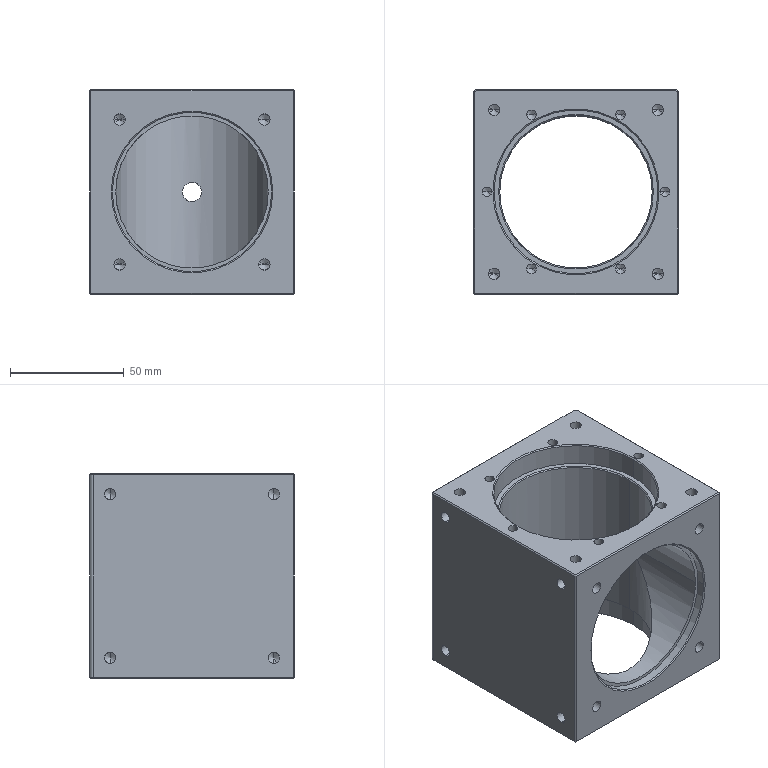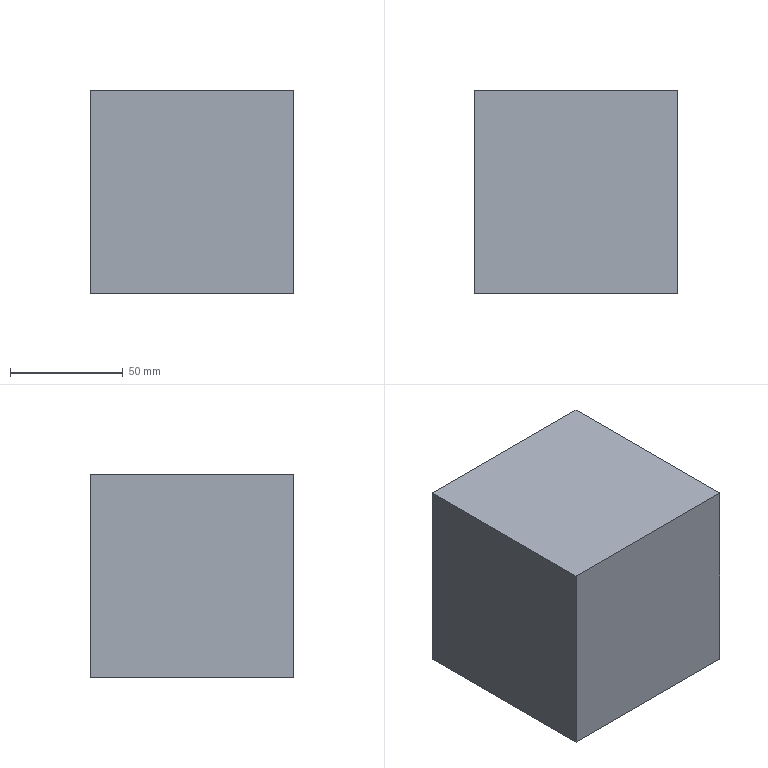CAM job | NX | 3+2 milling, drilling | part box 90 x 90 x 90 mm | stock box 90 x 90 x 90 mm
Tools:
number,name,description,diameter,corner_radius,flute_length,length,flutes
7,D6A45,Milling Tool-5 Parameters,6.0,0.0,3.0,3.0,2
14,4.2ZT,Drilling Tool,4.2,0.0,35.0,50.0,2
15,5.0ZT,Drilling Tool,5.0,0.0,35.0,50.0,2
9,9.0ZT,Drilling Tool,9.0,0.0,35.0,50.0,2
10,D10,Milling Tool-5 Parameters,10.0,0.0,50.0,75.0,2
16,D16,Milling Tool-5 Parameters,16.0,0.0,50.0,75.0,2
12,D12JING,Milling Tool-5 Parameters,12.0,0.0,50.0,75.0,2
Operations:
program,operation,operation_type,tool,method,geometry_group,spindle_rpm,surface_speed,feed_per_tooth,feed_cut,feed_plunge,cut_length_mm,path_length_mm,cut_time_min,machine_time_min
1,DRILLING_COPY_1_COPY_1,Operation,D6A45,METHOD,A,5000.0,94.0,0.025,250.0,0.0,20.0,329.62,0.08,0.111
1,DRILLING_COPY_1_COPY_COPY_COPY_COPY,Operation,5.0ZT,METHOD,A,2000.0,20.0,0.0375,150.0,0.0,86.009,432.148,0.5734,0.608
1,DRILLING_COPY_1_COPY_COPY_COPY_COPY_COPY,Operation,9.0ZT,METHOD,A,1200.0,33.0,0.0625,150.0,0.0,52.204,164.408,0.348,0.3592
1,HOLE_MILLING,CylinderMilling,D10,METHOD,A,9500.0,298.0,0.1158,2200.0,100.0,3013.112,3076.112,1.37,1.376
1,HOLE_MILLING_COPY,CylinderMilling,D16,METHOD,A,8500.0,427.0,0.1294,2200.0,100.0,5181.926,5289.926,2.355,2.366
1,HOLE_MILLING_COPY_COPY,CylinderMilling,D12JING,METHOD,A,8000.0,301.0,0.0625,1000.0,100.0,548.513,700.894,0.5485,0.5638
1,ZLEVEL_PROFILE_1_COPY_1_COPY,ZLevelMilling,D6A45,METHOD,A,9500.0,179.0,0.0526,1000.0,100.0,632.252,1243.393,0.6323,0.6934
2,DRILLING_COPY_1_COPY_1_COPY,Operation,D6A45,METHOD,B,5000.0,94.0,0.025,250.0,0.0,44.0,468.89,0.176,0.2185
2,DRILLING_COPY_1_COPY_COPY_COPY_COPY_COPY_1,Operation,5.0ZT,METHOD,B,2000.0,20.0,0.0375,150.0,0.0,56.473,398.134,0.3765,0.4107
2,DRILLING_COPY_1_COPY_COPY_COPY_COPY_COPY_1_COPY,Operation,4.2ZT,METHOD,B,2000.0,20.0,0.0375,150.0,0.0,109.571,490.216,0.7305,0.7685
2,DRILLING_COPY_1_COPY_COPY_COPY_COPY_COPY_COPY,Operation,9.0ZT,METHOD,B,1200.0,33.0,0.0625,150.0,0.0,52.704,165.408,0.3514,0.3626
2,HOLE_MILLING_COPY_1,CylinderMilling,D10,METHOD,B,9500.0,298.0,0.1158,2200.0,100.0,3303.902,3372.902,1.502,1.509
2,HOLE_MILLING_COPY_COPY_1,CylinderMilling,D16,METHOD,B,8500.0,427.0,0.1294,2200.0,100.0,5096.984,5212.484,2.317,2.328
2,HOLE_MILLING_COPY_COPY_COPY,CylinderMilling,D12JING,METHOD,B,8000.0,301.0,0.0625,1000.0,100.0,367.946,522.039,0.3679,0.3834
2,ZLEVEL_PROFILE_1_COPY_1_COPY_COPY,ZLevelMilling,D6A45,METHOD,B,9500.0,179.0,0.0526,1000.0,100.0,719.55,2099.199,0.7195,0.8575
3,DRILLING_COPY_1_COPY_1_COPY_COPY,Operation,D6A45,METHOD,C,5000.0,94.0,0.025,250.0,0.0,44.0,468.89,0.176,0.2185
3,DRILLING_COPY_1_COPY_COPY_COPY_COPY_COPY_1_COPY_1,Operation,5.0ZT,METHOD,C,2000.0,20.0,0.0375,150.0,0.0,56.473,398.134,0.3765,0.4107
3,DRILLING_COPY_1_COPY_COPY_COPY_COPY_COPY_1_COPY_COPY,Operation,4.2ZT,METHOD,C,2000.0,20.0,0.0375,150.0,0.0,109.571,490.216,0.7305,0.7685
3,DRILLING_COPY_1_COPY_COPY_COPY_COPY_COPY_COPY_COPY,Operation,9.0ZT,METHOD,C,1200.0,33.0,0.0625,150.0,0.0,52.704,165.408,0.3514,0.3626
3,HOLE_MILLING_COPY_1_COPY,CylinderMilling,D10,METHOD,C,9500.0,298.0,0.1158,2200.0,100.0,3303.902,3372.902,1.502,1.509
3,HOLE_MILLING_COPY_COPY_1_COPY,CylinderMilling,D16,METHOD,C,8500.0,427.0,0.1294,2200.0,100.0,5046.984,5164.484,2.294,2.306
3,HOLE_MILLING_COPY_COPY_COPY_COPY,CylinderMilling,D12JING,METHOD,C,8000.0,301.0,0.0625,1000.0,100.0,367.946,524.025,0.3679,0.3836
3,ZLEVEL_PROFILE_1_COPY_1_COPY_COPY_COPY,ZLevelMilling,D6A45,METHOD,C,9500.0,179.0,0.0526,1000.0,100.0,686.626,2046.34,0.6866,0.8226